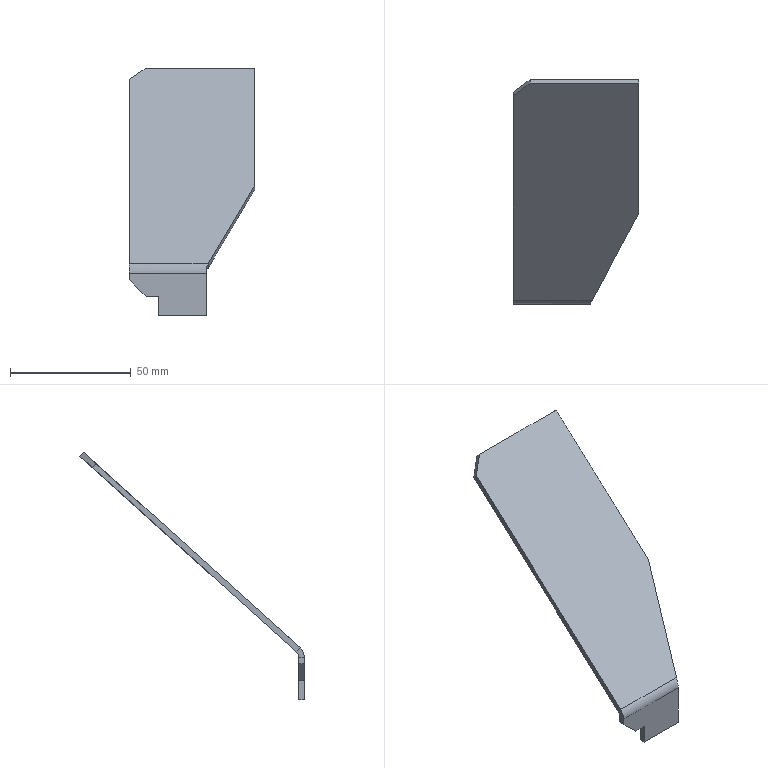Part | SolidWorks | features ICE 2, Chamfer 1, FlatPattern 1, SMBaseFlange 1, SheetMetal 1 | 1 solid | 20 faces | box 52 x 93.043 x 102.735 mm | volume 14624 mm3 | plane 17 | cylinder 2 | spline 1 | commonest cylinder face diameters 6 x1 10.6 x1
STEP:
#1=CARTESIAN_POINT('',(52.,37.522,53.927));
#2=VERTEX_POINT('',#1);
#3=CARTESIAN_POINT('',(52.,91.5,102.735));
#4=VERTEX_POINT('',#3);
#5=CARTESIAN_POINT('',(52.,0.,20.));
#6=DIRECTION('',(0.,0.7417,0.6707));
#7=VECTOR('',#6,1000.);
#8=LINE('',#5,#7);
#9=EDGE_CURVE('',#2,#4,#8,.T.);
#10=ORIENTED_EDGE('',*,*,#9,.F.);
#11=CARTESIAN_POINT('',(52.,39.065,52.221));
#12=VERTEX_POINT('',#11);
#13=CARTESIAN_POINT('',(52.,37.522,53.927));
#14=DIRECTION('',(0.,0.6707,-0.7417));
#15=VECTOR('',#14,1000.);
#16=LINE('',#13,#15);
#17=EDGE_CURVE('',#2,#12,#16,.T.);
#18=ORIENTED_EDGE('',*,*,#17,.T.);
#19=CARTESIAN_POINT('',(52.,93.043,101.029));
#20=VERTEX_POINT('',#19);
#21=CARTESIAN_POINT('',(52.,1.543,18.294));
#22=DIRECTION('',(0.,0.7417,0.6707));
#23=VECTOR('',#22,1000.);
#24=LINE('',#21,#23);
#25=EDGE_CURVE('',#12,#20,#24,.T.);
#26=ORIENTED_EDGE('',*,*,#25,.T.);
#27=CARTESIAN_POINT('',(52.,91.5,102.735));
#28=DIRECTION('',(0.,0.6707,-0.7417));
#29=VECTOR('',#28,1000.);
#30=LINE('',#27,#29);
#31=EDGE_CURVE('',#4,#20,#30,.T.);
#32=ORIENTED_EDGE('',*,*,#31,.F.);
#33=EDGE_LOOP('',(#10,#18,#26,#32));
#34=FACE_OUTER_BOUND('',#33,.T.);
#35=CARTESIAN_POINT('',(52.,2.3,17.647));
#36=DIRECTION('',(1.,0.,0.));
#37=DIRECTION('',(0.,0.,-1.));
#38=AXIS2_PLACEMENT_3D('',#35,#36,#37);
#39=PLANE('',#38);
#40=ADVANCED_FACE('',(#34),#39,.T.);
#41=CARTESIAN_POINT('',(0.,3.288,19.872));
#42=VERTEX_POINT('',#41);
#43=CARTESIAN_POINT('',(0.,87.85,96.334));
#44=VERTEX_POINT('',#43);
#45=CARTESIAN_POINT('',(0.,1.543,18.294));
#46=DIRECTION('',(0.,0.7417,0.6707));
#47=VECTOR('',#46,1000.);
#48=LINE('',#45,#47);
#49=EDGE_CURVE('',#42,#44,#48,.T.);
#50=ORIENTED_EDGE('',*,*,#49,.T.);
#51=CARTESIAN_POINT('',(7.,93.043,101.029));
#52=VERTEX_POINT('',#51);
#53=CARTESIAN_POINT('',(0.,87.85,96.334));
#54=DIRECTION('',(0.7071,0.5245,0.4742));
#55=VECTOR('',#54,1000.);
#56=LINE('',#53,#55);
#57=EDGE_CURVE('',#44,#52,#56,.T.);
#58=ORIENTED_EDGE('',*,*,#57,.T.);
#59=CARTESIAN_POINT('',(52.,93.043,101.029));
#60=DIRECTION('',(-1.,0.,0.));
#61=VECTOR('',#60,1000.);
#62=LINE('',#59,#61);
#63=EDGE_CURVE('',#20,#52,#62,.T.);
#64=ORIENTED_EDGE('',*,*,#63,.F.);
#65=ORIENTED_EDGE('',*,*,#25,.F.);
#66=CARTESIAN_POINT('',(32.707,3.288,19.872));
#67=VERTEX_POINT('',#66);
#68=CARTESIAN_POINT('',(32.,1.977,18.687));
#69=DIRECTION('',(-0.3714,-0.6887,-0.6227));
#70=VECTOR('',#69,1000.);
#71=LINE('',#68,#70);
#72=EDGE_CURVE('',#12,#67,#71,.T.);
#73=ORIENTED_EDGE('',*,*,#72,.T.);
#74=CARTESIAN_POINT('',(52.,3.288,19.872));
#75=DIRECTION('',(-1.,0.,0.));
#76=VECTOR('',#75,1000.);
#77=LINE('',#74,#76);
#78=EDGE_CURVE('',#67,#42,#77,.T.);
#79=ORIENTED_EDGE('',*,*,#78,.T.);
#80=EDGE_LOOP('',(#50,#58,#64,#65,#73,#79));
#81=FACE_OUTER_BOUND('',#80,.T.);
#82=CARTESIAN_POINT('',(52.,1.543,18.294));
#83=DIRECTION('',(0.,-0.6707,0.7417));
#84=DIRECTION('',(0.,-0.7417,-0.6707));
#85=AXIS2_PLACEMENT_3D('',#82,#83,#84);
#86=PLANE('',#85);
#87=ADVANCED_FACE('',(#81),#86,.F.);
#88=CARTESIAN_POINT('',(7.,91.5,102.735));
#89=VERTEX_POINT('',#88);
#90=CARTESIAN_POINT('',(52.,91.5,102.735));
#91=DIRECTION('',(-1.,0.,0.));
#92=VECTOR('',#91,1000.);
#93=LINE('',#90,#92);
#94=EDGE_CURVE('',#4,#89,#93,.T.);
#95=ORIENTED_EDGE('',*,*,#94,.T.);
#96=CARTESIAN_POINT('',(0.,86.308,98.04));
#97=VERTEX_POINT('',#96);
#98=CARTESIAN_POINT('',(-32.179,62.439,76.458));
#99=DIRECTION('',(-0.7071,-0.5245,-0.4742));
#100=VECTOR('',#99,1000.);
#101=LINE('',#98,#100);
#102=EDGE_CURVE('',#89,#97,#101,.T.);
#103=ORIENTED_EDGE('',*,*,#102,.T.);
#104=CARTESIAN_POINT('',(0.,1.745,21.578));
#105=VERTEX_POINT('',#104);
#106=CARTESIAN_POINT('',(0.,0.,20.));
#107=DIRECTION('',(0.,0.7417,0.6707));
#108=VECTOR('',#107,1000.);
#109=LINE('',#106,#108);
#110=EDGE_CURVE('',#105,#97,#109,.T.);
#111=ORIENTED_EDGE('',*,*,#110,.F.);
#112=CARTESIAN_POINT('',(32.707,1.745,21.578));
#113=VERTEX_POINT('',#112);
#114=CARTESIAN_POINT('',(52.,1.745,21.578));
#115=DIRECTION('',(-1.,0.,0.));
#116=VECTOR('',#115,1000.);
#117=LINE('',#114,#116);
#118=EDGE_CURVE('',#113,#105,#117,.T.);
#119=ORIENTED_EDGE('',*,*,#118,.F.);
#120=CARTESIAN_POINT('',(32.,0.4349,20.393));
#121=DIRECTION('',(-0.3714,-0.6887,-0.6227));
#122=VECTOR('',#121,1000.);
#123=LINE('',#120,#122);
#124=EDGE_CURVE('',#2,#113,#123,.T.);
#125=ORIENTED_EDGE('',*,*,#124,.F.);
#126=ORIENTED_EDGE('',*,*,#9,.T.);
#127=EDGE_LOOP('',(#95,#103,#111,#119,#125,#126));
#128=FACE_OUTER_BOUND('',#127,.T.);
#129=CARTESIAN_POINT('',(52.,0.,20.));
#130=DIRECTION('',(0.,-0.6707,0.7417));
#131=DIRECTION('',(0.,-0.7417,-0.6707));
#132=AXIS2_PLACEMENT_3D('',#129,#130,#131);
#133=PLANE('',#132);
#134=ADVANCED_FACE('',(#128),#133,.T.);
#135=CARTESIAN_POINT('',(32.,0.,17.647));
#136=VERTEX_POINT('',#135);
#137=CARTESIAN_POINT('',(0.,0.,17.647));
#138=VERTEX_POINT('',#137);
#139=CARTESIAN_POINT('',(52.,0.,17.647));
#140=DIRECTION('',(-1.,0.,0.));
#141=VECTOR('',#140,1000.);
#142=LINE('',#139,#141);
#143=EDGE_CURVE('',#136,#138,#142,.T.);
#144=ORIENTED_EDGE('',*,*,#143,.F.);
#145=CARTESIAN_POINT('',(32.,0.6382,20.168));
#146=VERTEX_POINT('',#145);
#147=CARTESIAN_POINT('',(32.,5.3,17.647));
#148=DIRECTION('',(1.,0.,0.));
#149=DIRECTION('',(0.,0.,1.));
#150=AXIS2_PLACEMENT_3D('',#147,#148,#149);
#151=CIRCLE('',#150,5.3);
#152=EDGE_CURVE('',#146,#136,#151,.T.);
#153=ORIENTED_EDGE('',*,*,#152,.F.);
#154=CARTESIAN_POINT('',(32.707,1.745,21.578));
#155=CARTESIAN_POINT('',(32.465,1.298,21.174));
#156=CARTESIAN_POINT('',(32.228,0.9252,20.699));
#157=CARTESIAN_POINT('',(32.,0.6382,20.168));
#158=(BOUNDED_CURVE()B_SPLINE_CURVE(3,(#154,#155,#156,#157),.UNSPECIFIED.,.F.,.T.)B_SPLINE_CURVE_WITH_KNOTS((4,4),(4.712,5.052),.UNSPECIFIED.)CURVE()GEOMETRIC_REPRESENTATION_ITEM()RATIONAL_B_SPLINE_CURVE((1.,0.9904,0.9904,1.))REPRESENTATION_ITEM(''));
#159=EDGE_CURVE('',#113,#146,#158,.T.);
#160=ORIENTED_EDGE('',*,*,#159,.F.);
#161=ORIENTED_EDGE('',*,*,#118,.T.);
#162=CARTESIAN_POINT('',(0.,5.3,17.647));
#163=DIRECTION('',(-1.,0.,0.));
#164=DIRECTION('',(0.,0.,-1.));
#165=AXIS2_PLACEMENT_3D('',#162,#163,#164);
#166=CIRCLE('',#165,5.3);
#167=EDGE_CURVE('',#138,#105,#166,.T.);
#168=ORIENTED_EDGE('',*,*,#167,.F.);
#169=EDGE_LOOP('',(#144,#153,#160,#161,#168));
#170=FACE_OUTER_BOUND('',#169,.T.);
#171=CARTESIAN_POINT('',(52.,5.3,17.647));
#172=DIRECTION('',(-1.,0.,0.));
#173=DIRECTION('',(0.,0.,1.));
#174=AXIS2_PLACEMENT_3D('',#171,#172,#173);
#175=CYLINDRICAL_SURFACE('',#174,5.3);
#176=ADVANCED_FACE('',(#170),#175,.T.);
#177=CARTESIAN_POINT('',(0.,0.,15.));
#178=VERTEX_POINT('',#177);
#179=CARTESIAN_POINT('',(0.,0.,0.));
#180=DIRECTION('',(0.,0.,1.));
#181=VECTOR('',#180,1000.);
#182=LINE('',#179,#181);
#183=EDGE_CURVE('',#178,#138,#182,.T.);
#184=ORIENTED_EDGE('',*,*,#183,.F.);
#185=CARTESIAN_POINT('',(7.,0.,8.));
#186=VERTEX_POINT('',#185);
#187=CARTESIAN_POINT('',(33.5,0.,-18.5));
#188=DIRECTION('',(0.7071,0.,-0.7071));
#189=VECTOR('',#188,1000.);
#190=LINE('',#187,#189);
#191=EDGE_CURVE('',#178,#186,#190,.T.);
#192=ORIENTED_EDGE('',*,*,#191,.T.);
#193=CARTESIAN_POINT('',(12.,0.,8.));
#194=VERTEX_POINT('',#193);
#195=CARTESIAN_POINT('',(12.,0.,8.));
#196=DIRECTION('',(-1.,0.,0.));
#197=VECTOR('',#196,1000.);
#198=LINE('',#195,#197);
#199=EDGE_CURVE('',#194,#186,#198,.T.);
#200=ORIENTED_EDGE('',*,*,#199,.F.);
#201=CARTESIAN_POINT('',(12.,0.,0.));
#202=VERTEX_POINT('',#201);
#203=CARTESIAN_POINT('',(12.,0.,0.));
#204=DIRECTION('',(0.,0.,1.));
#205=VECTOR('',#204,1000.);
#206=LINE('',#203,#205);
#207=EDGE_CURVE('',#202,#194,#206,.T.);
#208=ORIENTED_EDGE('',*,*,#207,.F.);
#209=CARTESIAN_POINT('',(32.,0.,0.));
#210=VERTEX_POINT('',#209);
#211=CARTESIAN_POINT('',(52.,0.,0.));
#212=DIRECTION('',(-1.,0.,0.));
#213=VECTOR('',#212,1000.);
#214=LINE('',#211,#213);
#215=EDGE_CURVE('',#210,#202,#214,.T.);
#216=ORIENTED_EDGE('',*,*,#215,.F.);
#217=CARTESIAN_POINT('',(32.,0.,0.));
#218=DIRECTION('',(0.,0.,-1.));
#219=VECTOR('',#218,1000.);
#220=LINE('',#217,#219);
#221=EDGE_CURVE('',#136,#210,#220,.T.);
#222=ORIENTED_EDGE('',*,*,#221,.F.);
#223=ORIENTED_EDGE('',*,*,#143,.T.);
#224=EDGE_LOOP('',(#184,#192,#200,#208,#216,#222,#223));
#225=FACE_OUTER_BOUND('',#224,.T.);
#226=CARTESIAN_POINT('',(52.,0.,0.));
#227=DIRECTION('',(0.,-1.,0.));
#228=DIRECTION('',(0.,0.,-1.));
#229=AXIS2_PLACEMENT_3D('',#226,#227,#228);
#230=PLANE('',#229);
#231=ADVANCED_FACE('',(#225),#230,.T.);
#232=CARTESIAN_POINT('',(32.,2.3,0.));
#233=VERTEX_POINT('',#232);
#234=CARTESIAN_POINT('',(12.,2.3,0.));
#235=VERTEX_POINT('',#234);
#236=CARTESIAN_POINT('',(52.,2.3,0.));
#237=DIRECTION('',(-1.,0.,0.));
#238=VECTOR('',#237,1000.);
#239=LINE('',#236,#238);
#240=EDGE_CURVE('',#233,#235,#239,.T.);
#241=ORIENTED_EDGE('',*,*,#240,.F.);
#242=CARTESIAN_POINT('',(32.,2.3,0.));
#243=DIRECTION('',(0.,-1.,0.));
#244=VECTOR('',#243,1000.);
#245=LINE('',#242,#244);
#246=EDGE_CURVE('',#233,#210,#245,.T.);
#247=ORIENTED_EDGE('',*,*,#246,.T.);
#248=ORIENTED_EDGE('',*,*,#215,.T.);
#249=CARTESIAN_POINT('',(12.,93.044,0.));
#250=DIRECTION('',(0.,-1.,0.));
#251=VECTOR('',#250,1000.);
#252=LINE('',#249,#251);
#253=EDGE_CURVE('',#235,#202,#252,.T.);
#254=ORIENTED_EDGE('',*,*,#253,.F.);
#255=EDGE_LOOP('',(#241,#247,#248,#254));
#256=FACE_OUTER_BOUND('',#255,.T.);
#257=CARTESIAN_POINT('',(52.,2.3,0.));
#258=DIRECTION('',(0.,0.,-1.));
#259=DIRECTION('',(-1.,0.,0.));
#260=AXIS2_PLACEMENT_3D('',#257,#258,#259);
#261=PLANE('',#260);
#262=ADVANCED_FACE('',(#256),#261,.T.);
#263=CARTESIAN_POINT('',(7.,2.3,8.));
#264=VERTEX_POINT('',#263);
#265=CARTESIAN_POINT('',(12.,2.3,8.));
#266=VERTEX_POINT('',#265);
#267=CARTESIAN_POINT('',(12.,2.3,8.));
#268=DIRECTION('',(1.,0.,0.));
#269=VECTOR('',#268,1000.);
#270=LINE('',#267,#269);
#271=EDGE_CURVE('',#264,#266,#270,.T.);
#272=ORIENTED_EDGE('',*,*,#271,.F.);
#273=CARTESIAN_POINT('',(0.,2.3,15.));
#274=VERTEX_POINT('',#273);
#275=CARTESIAN_POINT('',(0.,2.3,15.));
#276=DIRECTION('',(-0.7071,0.,0.7071));
#277=VECTOR('',#276,1000.);
#278=LINE('',#275,#277);
#279=EDGE_CURVE('',#264,#274,#278,.T.);
#280=ORIENTED_EDGE('',*,*,#279,.T.);
#281=CARTESIAN_POINT('',(0.,2.3,17.647));
#282=VERTEX_POINT('',#281);
#283=CARTESIAN_POINT('',(0.,2.3,0.));
#284=DIRECTION('',(0.,0.,1.));
#285=VECTOR('',#284,1000.);
#286=LINE('',#283,#285);
#287=EDGE_CURVE('',#274,#282,#286,.T.);
#288=ORIENTED_EDGE('',*,*,#287,.T.);
#289=CARTESIAN_POINT('',(32.,2.3,17.647));
#290=VERTEX_POINT('',#289);
#291=CARTESIAN_POINT('',(52.,2.3,17.647));
#292=DIRECTION('',(-1.,0.,0.));
#293=VECTOR('',#292,1000.);
#294=LINE('',#291,#293);
#295=EDGE_CURVE('',#290,#282,#294,.T.);
#296=ORIENTED_EDGE('',*,*,#295,.F.);
#297=CARTESIAN_POINT('',(32.,2.3,0.));
#298=DIRECTION('',(0.,0.,-1.));
#299=VECTOR('',#298,1000.);
#300=LINE('',#297,#299);
#301=EDGE_CURVE('',#290,#233,#300,.T.);
#302=ORIENTED_EDGE('',*,*,#301,.T.);
#303=ORIENTED_EDGE('',*,*,#240,.T.);
#304=CARTESIAN_POINT('',(12.,2.3,0.));
#305=DIRECTION('',(0.,0.,-1.));
#306=VECTOR('',#305,1000.);
#307=LINE('',#304,#306);
#308=EDGE_CURVE('',#266,#235,#307,.T.);
#309=ORIENTED_EDGE('',*,*,#308,.F.);
#310=EDGE_LOOP('',(#272,#280,#288,#296,#302,#303,#309));
#311=FACE_OUTER_BOUND('',#310,.T.);
#312=CARTESIAN_POINT('',(52.,2.3,0.));
#313=DIRECTION('',(0.,-1.,0.));
#314=DIRECTION('',(0.,0.,-1.));
#315=AXIS2_PLACEMENT_3D('',#312,#313,#314);
#316=PLANE('',#315);
#317=ADVANCED_FACE('',(#311),#316,.F.);
#318=CARTESIAN_POINT('',(32.,2.661,19.074));
#319=VERTEX_POINT('',#318);
#320=CARTESIAN_POINT('',(32.,5.3,17.647));
#321=DIRECTION('',(1.,0.,0.));
#322=DIRECTION('',(0.,0.,1.));
#323=AXIS2_PLACEMENT_3D('',#320,#321,#322);
#324=CIRCLE('',#323,3.);
#325=EDGE_CURVE('',#319,#290,#324,.T.);
#326=ORIENTED_EDGE('',*,*,#325,.T.);
#327=ORIENTED_EDGE('',*,*,#295,.T.);
#328=CARTESIAN_POINT('',(0.,5.3,17.647));
#329=DIRECTION('',(-1.,0.,0.));
#330=DIRECTION('',(0.,0.,-1.));
#331=AXIS2_PLACEMENT_3D('',#328,#329,#330);
#332=CIRCLE('',#331,3.);
#333=EDGE_CURVE('',#282,#42,#332,.T.);
#334=ORIENTED_EDGE('',*,*,#333,.T.);
#335=ORIENTED_EDGE('',*,*,#78,.F.);
#336=CARTESIAN_POINT('',(32.707,3.288,19.872));
#337=CARTESIAN_POINT('',(32.465,3.035,19.643));
#338=CARTESIAN_POINT('',(32.228,2.824,19.375));
#339=CARTESIAN_POINT('',(32.,2.661,19.074));
#340=(BOUNDED_CURVE()B_SPLINE_CURVE(3,(#336,#337,#338,#339),.UNSPECIFIED.,.F.,.T.)B_SPLINE_CURVE_WITH_KNOTS((4,4),(4.712,5.052),.UNSPECIFIED.)CURVE()GEOMETRIC_REPRESENTATION_ITEM()RATIONAL_B_SPLINE_CURVE((1.,0.9904,0.9904,1.))REPRESENTATION_ITEM(''));
#341=EDGE_CURVE('',#67,#319,#340,.T.);
#342=ORIENTED_EDGE('',*,*,#341,.T.);
#343=EDGE_LOOP('',(#326,#327,#334,#335,#342));
#344=FACE_OUTER_BOUND('',#343,.T.);
#345=CARTESIAN_POINT('',(52.,5.3,17.647));
#346=DIRECTION('',(-1.,0.,0.));
#347=DIRECTION('',(0.,0.,1.));
#348=AXIS2_PLACEMENT_3D('',#345,#346,#347);
#349=CYLINDRICAL_SURFACE('',#348,3.);
#350=ADVANCED_FACE('',(#344),#349,.F.);
#351=CARTESIAN_POINT('',(0.,0.,17.647));
#352=DIRECTION('',(0.,1.,0.));
#353=VECTOR('',#352,1000.);
#354=LINE('',#351,#353);
#355=EDGE_CURVE('',#138,#282,#354,.T.);
#356=ORIENTED_EDGE('',*,*,#355,.F.);
#357=ORIENTED_EDGE('',*,*,#167,.T.);
#358=CARTESIAN_POINT('',(0.,3.288,19.872));
#359=DIRECTION('',(0.,-0.6707,0.7417));
#360=VECTOR('',#359,1000.);
#361=LINE('',#358,#360);
#362=EDGE_CURVE('',#42,#105,#361,.T.);
#363=ORIENTED_EDGE('',*,*,#362,.F.);
#364=ORIENTED_EDGE('',*,*,#333,.F.);
#365=EDGE_LOOP('',(#356,#357,#363,#364));
#366=FACE_OUTER_BOUND('',#365,.T.);
#367=CARTESIAN_POINT('',(0.,0.,17.647));
#368=DIRECTION('',(-1.,0.,0.));
#369=DIRECTION('',(0.,0.,1.));
#370=AXIS2_PLACEMENT_3D('',#367,#368,#369);
#371=PLANE('',#370);
#372=ADVANCED_FACE('',(#366),#371,.T.);
#373=ORIENTED_EDGE('',*,*,#287,.F.);
#374=CARTESIAN_POINT('',(0.,0.,15.));
#375=DIRECTION('',(0.,-1.,0.));
#376=VECTOR('',#375,1000.);
#377=LINE('',#374,#376);
#378=EDGE_CURVE('',#274,#178,#377,.T.);
#379=ORIENTED_EDGE('',*,*,#378,.T.);
#380=ORIENTED_EDGE('',*,*,#183,.T.);
#381=ORIENTED_EDGE('',*,*,#355,.T.);
#382=EDGE_LOOP('',(#373,#379,#380,#381));
#383=FACE_OUTER_BOUND('',#382,.T.);
#384=CARTESIAN_POINT('',(0.,3.288,19.872));
#385=DIRECTION('',(-1.,0.,0.));
#386=DIRECTION('',(0.,0.,1.));
#387=AXIS2_PLACEMENT_3D('',#384,#385,#386);
#388=PLANE('',#387);
#389=ADVANCED_FACE('',(#383),#388,.T.);
#390=ORIENTED_EDGE('',*,*,#63,.T.);
#391=CARTESIAN_POINT('',(7.,91.5,102.735));
#392=DIRECTION('',(0.,-0.6707,0.7417));
#393=VECTOR('',#392,1000.);
#394=LINE('',#391,#393);
#395=EDGE_CURVE('',#52,#89,#394,.T.);
#396=ORIENTED_EDGE('',*,*,#395,.T.);
#397=ORIENTED_EDGE('',*,*,#94,.F.);
#398=ORIENTED_EDGE('',*,*,#31,.T.);
#399=EDGE_LOOP('',(#390,#396,#397,#398));
#400=FACE_OUTER_BOUND('',#399,.T.);
#401=CARTESIAN_POINT('',(52.,91.5,102.735));
#402=DIRECTION('',(0.,0.7417,0.6707));
#403=DIRECTION('',(0.,-0.6707,0.7417));
#404=AXIS2_PLACEMENT_3D('',#401,#402,#403);
#405=PLANE('',#404);
#406=ADVANCED_FACE('',(#400),#405,.T.);
#407=ORIENTED_EDGE('',*,*,#110,.T.);
#408=CARTESIAN_POINT('',(0.,87.85,96.334));
#409=DIRECTION('',(0.,0.6707,-0.7417));
#410=VECTOR('',#409,1000.);
#411=LINE('',#408,#410);
#412=EDGE_CURVE('',#97,#44,#411,.T.);
#413=ORIENTED_EDGE('',*,*,#412,.T.);
#414=ORIENTED_EDGE('',*,*,#49,.F.);
#415=ORIENTED_EDGE('',*,*,#362,.T.);
#416=EDGE_LOOP('',(#407,#413,#414,#415));
#417=FACE_OUTER_BOUND('',#416,.T.);
#418=CARTESIAN_POINT('',(0.,5.3,17.647));
#419=DIRECTION('',(1.,0.,0.));
#420=DIRECTION('',(0.,0.,-1.));
#421=AXIS2_PLACEMENT_3D('',#418,#419,#420);
#422=PLANE('',#421);
#423=ADVANCED_FACE('',(#417),#422,.F.);
#424=ORIENTED_EDGE('',*,*,#199,.T.);
#425=CARTESIAN_POINT('',(7.,2.3,8.));
#426=DIRECTION('',(0.,1.,0.));
#427=VECTOR('',#426,1000.);
#428=LINE('',#425,#427);
#429=EDGE_CURVE('',#186,#264,#428,.T.);
#430=ORIENTED_EDGE('',*,*,#429,.T.);
#431=ORIENTED_EDGE('',*,*,#271,.T.);
#432=CARTESIAN_POINT('',(12.,93.044,8.));
#433=DIRECTION('',(0.,-1.,0.));
#434=VECTOR('',#433,1000.);
#435=LINE('',#432,#434);
#436=EDGE_CURVE('',#266,#194,#435,.T.);
#437=ORIENTED_EDGE('',*,*,#436,.T.);
#438=EDGE_LOOP('',(#424,#430,#431,#437));
#439=FACE_OUTER_BOUND('',#438,.T.);
#440=CARTESIAN_POINT('',(12.,93.044,8.));
#441=DIRECTION('',(0.,0.,1.));
#442=DIRECTION('',(1.,0.,0.));
#443=AXIS2_PLACEMENT_3D('',#440,#441,#442);
#444=PLANE('',#443);
#445=ADVANCED_FACE('',(#439),#444,.F.);
#446=ORIENTED_EDGE('',*,*,#308,.T.);
#447=ORIENTED_EDGE('',*,*,#253,.T.);
#448=ORIENTED_EDGE('',*,*,#207,.T.);
#449=ORIENTED_EDGE('',*,*,#436,.F.);
#450=EDGE_LOOP('',(#446,#447,#448,#449));
#451=FACE_OUTER_BOUND('',#450,.T.);
#452=CARTESIAN_POINT('',(12.,93.044,0.));
#453=DIRECTION('',(1.,0.,0.));
#454=DIRECTION('',(0.,0.,-1.));
#455=AXIS2_PLACEMENT_3D('',#452,#453,#454);
#456=PLANE('',#455);
#457=ADVANCED_FACE('',(#451),#456,.F.);
#458=ORIENTED_EDGE('',*,*,#124,.T.);
#459=CARTESIAN_POINT('',(32.707,1.745,21.578));
#460=DIRECTION('',(0.,0.6707,-0.7417));
#461=VECTOR('',#460,1000.);
#462=LINE('',#459,#461);
#463=EDGE_CURVE('',#113,#67,#462,.T.);
#464=ORIENTED_EDGE('',*,*,#463,.T.);
#465=ORIENTED_EDGE('',*,*,#72,.F.);
#466=ORIENTED_EDGE('',*,*,#17,.F.);
#467=EDGE_LOOP('',(#458,#464,#465,#466));
#468=FACE_OUTER_BOUND('',#467,.T.);
#469=CARTESIAN_POINT('',(32.,0.4349,20.393));
#470=DIRECTION('',(-0.9285,0.2755,0.2491));
#471=DIRECTION('',(-0.3714,-0.6887,-0.6227));
#472=AXIS2_PLACEMENT_3D('',#469,#470,#471);
#473=PLANE('',#472);
#474=ADVANCED_FACE('',(#468),#473,.F.);
#475=ORIENTED_EDGE('',*,*,#246,.F.);
#476=ORIENTED_EDGE('',*,*,#301,.F.);
#477=CARTESIAN_POINT('',(32.,2.3,17.647));
#478=DIRECTION('',(0.,-1.,0.));
#479=VECTOR('',#478,1000.);
#480=LINE('',#477,#479);
#481=EDGE_CURVE('',#290,#136,#480,.T.);
#482=ORIENTED_EDGE('',*,*,#481,.T.);
#483=ORIENTED_EDGE('',*,*,#221,.T.);
#484=EDGE_LOOP('',(#475,#476,#482,#483));
#485=FACE_OUTER_BOUND('',#484,.T.);
#486=CARTESIAN_POINT('',(32.,2.3,0.));
#487=DIRECTION('',(-1.,0.,0.));
#488=DIRECTION('',(0.,0.,-1.));
#489=AXIS2_PLACEMENT_3D('',#486,#487,#488);
#490=PLANE('',#489);
#491=ADVANCED_FACE('',(#485),#490,.F.);
#492=ORIENTED_EDGE('',*,*,#481,.F.);
#493=ORIENTED_EDGE('',*,*,#325,.F.);
#494=CARTESIAN_POINT('',(32.,0.6382,20.168));
#495=DIRECTION('',(0.,0.8796,-0.4757));
#496=VECTOR('',#495,1000.);
#497=LINE('',#494,#496);
#498=EDGE_CURVE('',#146,#319,#497,.T.);
#499=ORIENTED_EDGE('',*,*,#498,.F.);
#500=ORIENTED_EDGE('',*,*,#152,.T.);
#501=EDGE_LOOP('',(#492,#493,#499,#500));
#502=FACE_OUTER_BOUND('',#501,.T.);
#503=CARTESIAN_POINT('',(32.,5.3,17.647));
#504=DIRECTION('',(1.,0.,0.));
#505=DIRECTION('',(0.,0.,-1.));
#506=AXIS2_PLACEMENT_3D('',#503,#504,#505);
#507=PLANE('',#506);
#508=ADVANCED_FACE('',(#502),#507,.T.);
#509=ORIENTED_EDGE('',*,*,#159,.T.);
#510=ORIENTED_EDGE('',*,*,#498,.T.);
#511=ORIENTED_EDGE('',*,*,#341,.F.);
#512=ORIENTED_EDGE('',*,*,#463,.F.);
#513=EDGE_LOOP('',(#509,#510,#511,#512));
#514=FACE_OUTER_BOUND('',#513,.T.);
#515=CARTESIAN_POINT('',(30.587,1.369,14.092));
#516=CARTESIAN_POINT('',(30.587,1.937,14.606));
#517=CARTESIAN_POINT('',(30.587,2.506,15.121));
#518=CARTESIAN_POINT('',(30.587,3.075,15.635));
#519=CARTESIAN_POINT('',(30.587,8.478,6.23));
#520=CARTESIAN_POINT('',(30.587,8.018,7.881));
#521=CARTESIAN_POINT('',(30.587,7.559,9.533));
#522=CARTESIAN_POINT('',(30.587,7.099,11.184));
#523=CARTESIAN_POINT('',(34.827,16.34,13.339));
#524=CARTESIAN_POINT('',(34.827,14.743,13.962));
#525=CARTESIAN_POINT('',(34.827,13.146,14.585));
#526=CARTESIAN_POINT('',(34.827,11.549,15.209));
#527=CARTESIAN_POINT('',(34.827,9.231,21.202));
#528=CARTESIAN_POINT('',(34.827,8.663,20.687));
#529=CARTESIAN_POINT('',(34.827,8.094,20.173));
#530=CARTESIAN_POINT('',(34.827,7.525,19.659));
#531=CARTESIAN_POINT('',(34.827,2.122,29.064));
#532=CARTESIAN_POINT('',(34.827,2.582,27.413));
#533=CARTESIAN_POINT('',(34.827,3.041,25.761));
#534=CARTESIAN_POINT('',(34.827,3.501,24.109));
#535=CARTESIAN_POINT('',(30.587,-5.74,21.955));
#536=CARTESIAN_POINT('',(30.587,-4.143,21.332));
#537=CARTESIAN_POINT('',(30.587,-2.546,20.708));
#538=CARTESIAN_POINT('',(30.587,-0.9493,20.085));
#539=CARTESIAN_POINT('',(30.587,1.369,14.092));
#540=CARTESIAN_POINT('',(30.587,1.937,14.606));
#541=CARTESIAN_POINT('',(30.587,2.506,15.121));
#542=CARTESIAN_POINT('',(30.587,3.075,15.635));
#543=(BOUNDED_SURFACE()B_SPLINE_SURFACE(3,3,((#515,#516,#517,#518),(#519,#520,#521,#522),(#523,#524,#525,#526),(#527,#528,#529,#530),(#531,#532,#533,#534),(#535,#536,#537,#538),(#539,#540,#541,#542)),.UNSPECIFIED.,.T.,.F.,.F.)B_SPLINE_SURFACE_WITH_KNOTS((4,3,4),(4,4),(0.,0.5,1.),(0.,1.),.UNSPECIFIED.)GEOMETRIC_REPRESENTATION_ITEM()RATIONAL_B_SPLINE_SURFACE(((1.,1.,1.,1.),(0.3333,0.3333,0.3333,0.3333),(0.3333,0.3333,0.3333,0.3333),(1.,1.,1.,1.),(0.3333,0.3333,0.3333,0.3333),(0.3333,0.3333,0.3333,0.3333),(1.,1.,1.,1.)))REPRESENTATION_ITEM('')SURFACE());
#544=ADVANCED_FACE('',(#514),#543,.T.);
#545=ORIENTED_EDGE('',*,*,#102,.F.);
#546=ORIENTED_EDGE('',*,*,#395,.F.);
#547=ORIENTED_EDGE('',*,*,#57,.F.);
#548=ORIENTED_EDGE('',*,*,#412,.F.);
#549=EDGE_LOOP('',(#545,#546,#547,#548));
#550=FACE_OUTER_BOUND('',#549,.T.);
#551=CARTESIAN_POINT('',(0.,89.862,94.109));
#552=DIRECTION('',(-0.7071,0.5245,0.4742));
#553=DIRECTION('',(0.,-0.6707,0.7417));
#554=AXIS2_PLACEMENT_3D('',#551,#552,#553);
#555=PLANE('',#554);
#556=ADVANCED_FACE('',(#550),#555,.T.);
#557=ORIENTED_EDGE('',*,*,#279,.F.);
#558=ORIENTED_EDGE('',*,*,#429,.F.);
#559=ORIENTED_EDGE('',*,*,#191,.F.);
#560=ORIENTED_EDGE('',*,*,#378,.F.);
#561=EDGE_LOOP('',(#557,#558,#559,#560));
#562=FACE_OUTER_BOUND('',#561,.T.);
#563=CARTESIAN_POINT('',(0.,3.288,15.));
#564=DIRECTION('',(-0.7071,0.,-0.7071));
#565=DIRECTION('',(0.,1.,0.));
#566=AXIS2_PLACEMENT_3D('',#563,#564,#565);
#567=PLANE('',#566);
#568=ADVANCED_FACE('',(#562),#567,.T.);
#569=CLOSED_SHELL('',(#40,#87,#134,#176,#231,#262,#317,#350,#372,#389,#406,#423,#445,#457,#474,#491,#508,#544,#556,#568));
#570=MANIFOLD_SOLID_BREP('',#569);
#571=CARTESIAN_POINT('',(0.,0.,0.));
#572=DIRECTION('',(0.,0.,1.));
#573=DIRECTION('',(1.,0.,0.));
#574=AXIS2_PLACEMENT_3D('',#571,#572,#573);
#575=(LENGTH_UNIT()NAMED_UNIT(*)SI_UNIT(.MILLI.,.METRE.));
#576=UNCERTAINTY_MEASURE_WITH_UNIT(LENGTH_MEASURE(0.00001),#575,'','');
#577=(NAMED_UNIT(*)PLANE_ANGLE_UNIT()SI_UNIT($,.RADIAN.));
#578=(NAMED_UNIT(*)SI_UNIT($,.STERADIAN.)SOLID_ANGLE_UNIT());
#579=(GEOMETRIC_REPRESENTATION_CONTEXT(3)GLOBAL_UNCERTAINTY_ASSIGNED_CONTEXT((#576))GLOBAL_UNIT_ASSIGNED_CONTEXT((#575,#577,#578))REPRESENTATION_CONTEXT('',''));
#580=ADVANCED_BREP_SHAPE_REPRESENTATION('',(#570,#574),#579);